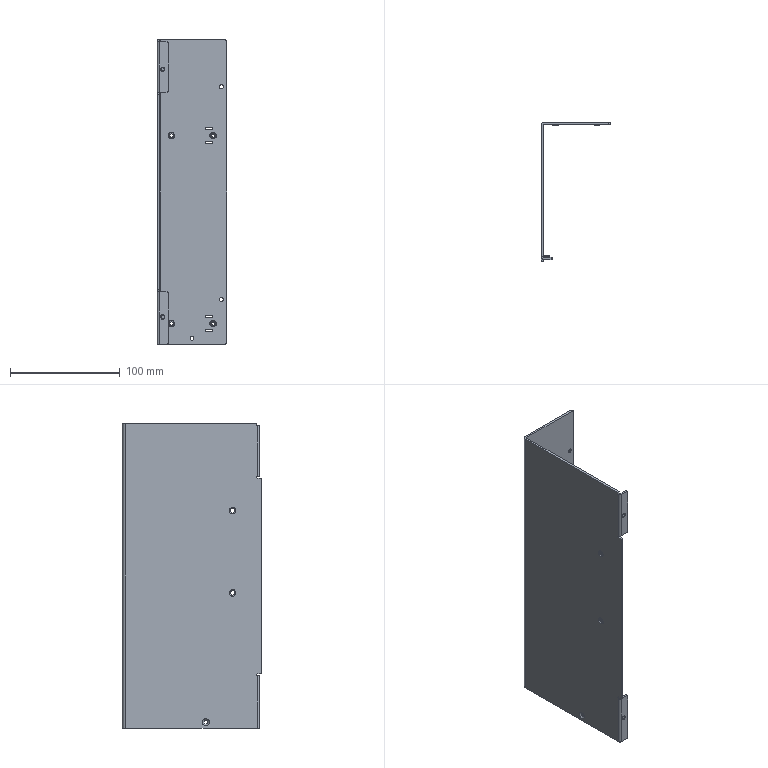Part | NX | features BREP 1 | 1 solid | 90 faces | box 63.5 x 127 x 278 mm | volume 104964 mm3 | plane 42 | cylinder 30 | torus 12 | cone 6 | commonest cylinder face diameters 2 x7 3 x6 5 x6 3.5 x4 4 x4 4.3 x2